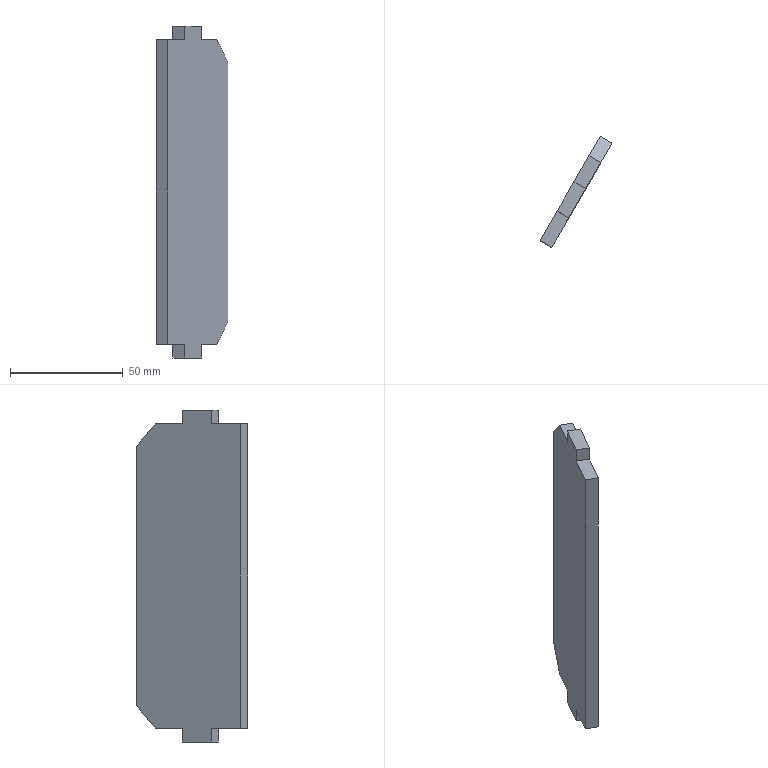Part | SolidWorks | features SMBaseFlange 2, Chamfer 1, FlatPattern 1, SheetMetal 1 | 1 solid | 16 faces | box 31.874 x 49.208 x 147 mm | volume 43699 mm3 | plane 16
STEP:
#1=CARTESIAN_POINT('',(44.488,-29.227,135.));
#2=VERTEX_POINT('',#1);
#3=CARTESIAN_POINT('',(39.291,-26.227,135.));
#4=VERTEX_POINT('',#3);
#5=CARTESIAN_POINT('',(44.488,-29.227,135.));
#6=DIRECTION('',(-0.866,0.5,0.));
#7=VECTOR('',#6,1000.);
#8=LINE('',#5,#7);
#9=EDGE_CURVE('',#2,#4,#8,.T.);
#10=ORIENTED_EDGE('',*,*,#9,.F.);
#11=CARTESIAN_POINT('',(51.166,-17.66,135.));
#12=VERTEX_POINT('',#11);
#13=CARTESIAN_POINT('',(29.488,-55.208,135.));
#14=DIRECTION('',(0.5,0.866,0.));
#15=VECTOR('',#14,1000.);
#16=LINE('',#13,#15);
#17=EDGE_CURVE('',#2,#12,#16,.T.);
#18=ORIENTED_EDGE('',*,*,#17,.T.);
#19=CARTESIAN_POINT('',(45.97,-14.66,135.));
#20=VERTEX_POINT('',#19);
#21=CARTESIAN_POINT('',(45.97,-14.66,135.));
#22=DIRECTION('',(-0.866,0.5,0.));
#23=VECTOR('',#22,1000.);
#24=LINE('',#21,#23);
#25=EDGE_CURVE('',#12,#20,#24,.T.);
#26=ORIENTED_EDGE('',*,*,#25,.T.);
#27=CARTESIAN_POINT('',(24.291,-52.208,135.));
#28=DIRECTION('',(0.5,0.866,0.));
#29=VECTOR('',#28,1000.);
#30=LINE('',#27,#29);
#31=EDGE_CURVE('',#4,#20,#30,.T.);
#32=ORIENTED_EDGE('',*,*,#31,.F.);
#33=EDGE_LOOP('',(#10,#18,#26,#32));
#34=FACE_OUTER_BOUND('',#33,.T.);
#35=CARTESIAN_POINT('',(0.,0.,135.));
#36=DIRECTION('',(0.,0.,-1.));
#37=DIRECTION('',(-1.,0.,0.));
#38=AXIS2_PLACEMENT_3D('',#35,#36,#37);
#39=PLANE('',#38);
#40=ADVANCED_FACE('',(#34),#39,.F.);
#41=CARTESIAN_POINT('',(44.488,-29.227,0.));
#42=VERTEX_POINT('',#41);
#43=CARTESIAN_POINT('',(51.166,-17.66,0.));
#44=VERTEX_POINT('',#43);
#45=CARTESIAN_POINT('',(29.488,-55.208,0.));
#46=DIRECTION('',(0.5,0.866,0.));
#47=VECTOR('',#46,1000.);
#48=LINE('',#45,#47);
#49=EDGE_CURVE('',#42,#44,#48,.T.);
#50=ORIENTED_EDGE('',*,*,#49,.F.);
#51=CARTESIAN_POINT('',(39.291,-26.227,0.));
#52=VERTEX_POINT('',#51);
#53=CARTESIAN_POINT('',(44.488,-29.227,0.));
#54=DIRECTION('',(-0.866,0.5,0.));
#55=VECTOR('',#54,1000.);
#56=LINE('',#53,#55);
#57=EDGE_CURVE('',#42,#52,#56,.T.);
#58=ORIENTED_EDGE('',*,*,#57,.T.);
#59=CARTESIAN_POINT('',(45.97,-14.66,0.));
#60=VERTEX_POINT('',#59);
#61=CARTESIAN_POINT('',(24.291,-52.208,0.));
#62=DIRECTION('',(0.5,0.866,0.));
#63=VECTOR('',#62,1000.);
#64=LINE('',#61,#63);
#65=EDGE_CURVE('',#52,#60,#64,.T.);
#66=ORIENTED_EDGE('',*,*,#65,.T.);
#67=CARTESIAN_POINT('',(5.144,8.91,0.));
#68=DIRECTION('',(0.866,-0.5,0.));
#69=VECTOR('',#68,1000.);
#70=LINE('',#67,#69);
#71=EDGE_CURVE('',#60,#44,#70,.T.);
#72=ORIENTED_EDGE('',*,*,#71,.T.);
#73=EDGE_LOOP('',(#50,#58,#66,#72));
#74=FACE_OUTER_BOUND('',#73,.T.);
#75=CARTESIAN_POINT('',(0.,0.,0.));
#76=DIRECTION('',(0.,0.,-1.));
#77=DIRECTION('',(-1.,0.,0.));
#78=AXIS2_PLACEMENT_3D('',#75,#76,#77);
#79=PLANE('',#78);
#80=ADVANCED_FACE('',(#74),#79,.T.);
#81=CARTESIAN_POINT('',(56.166,-9.,125.));
#82=VERTEX_POINT('',#81);
#83=CARTESIAN_POINT('',(56.166,-9.,10.));
#84=VERTEX_POINT('',#83);
#85=CARTESIAN_POINT('',(56.166,-9.,135.));
#86=DIRECTION('',(0.,0.,-1.));
#87=VECTOR('',#86,1000.);
#88=LINE('',#85,#87);
#89=EDGE_CURVE('',#82,#84,#88,.T.);
#90=ORIENTED_EDGE('',*,*,#89,.F.);
#91=CARTESIAN_POINT('',(56.166,-9.,125.));
#92=DIRECTION('',(-0.3536,-0.6124,0.7071));
#93=VECTOR('',#92,1000.);
#94=LINE('',#91,#93);
#95=EDGE_CURVE('',#82,#12,#94,.T.);
#96=ORIENTED_EDGE('',*,*,#95,.T.);
#97=ORIENTED_EDGE('',*,*,#17,.F.);
#98=CARTESIAN_POINT('',(44.488,-29.227,141.));
#99=VERTEX_POINT('',#98);
#100=CARTESIAN_POINT('',(44.488,-29.227,135.));
#101=DIRECTION('',(0.,0.,-1.));
#102=VECTOR('',#101,1000.);
#103=LINE('',#100,#102);
#104=EDGE_CURVE('',#99,#2,#103,.T.);
#105=ORIENTED_EDGE('',*,*,#104,.F.);
#106=CARTESIAN_POINT('',(36.988,-42.218,141.));
#107=VERTEX_POINT('',#106);
#108=CARTESIAN_POINT('',(44.488,-29.227,141.));
#109=DIRECTION('',(0.5,0.866,0.));
#110=VECTOR('',#109,1000.);
#111=LINE('',#108,#110);
#112=EDGE_CURVE('',#107,#99,#111,.T.);
#113=ORIENTED_EDGE('',*,*,#112,.F.);
#114=CARTESIAN_POINT('',(36.988,-42.218,135.));
#115=VERTEX_POINT('',#114);
#116=CARTESIAN_POINT('',(36.988,-42.218,141.));
#117=DIRECTION('',(0.,0.,1.));
#118=VECTOR('',#117,1000.);
#119=LINE('',#116,#118);
#120=EDGE_CURVE('',#115,#107,#119,.T.);
#121=ORIENTED_EDGE('',*,*,#120,.F.);
#122=CARTESIAN_POINT('',(29.488,-55.208,135.));
#123=VERTEX_POINT('',#122);
#124=CARTESIAN_POINT('',(29.488,-55.208,135.));
#125=DIRECTION('',(0.5,0.866,0.));
#126=VECTOR('',#125,1000.);
#127=LINE('',#124,#126);
#128=EDGE_CURVE('',#123,#115,#127,.T.);
#129=ORIENTED_EDGE('',*,*,#128,.F.);
#130=CARTESIAN_POINT('',(29.488,-55.208,0.));
#131=VERTEX_POINT('',#130);
#132=CARTESIAN_POINT('',(29.488,-55.208,135.));
#133=DIRECTION('',(0.,0.,-1.));
#134=VECTOR('',#133,1000.);
#135=LINE('',#132,#134);
#136=EDGE_CURVE('',#123,#131,#135,.T.);
#137=ORIENTED_EDGE('',*,*,#136,.T.);
#138=CARTESIAN_POINT('',(36.988,-42.218,0.));
#139=VERTEX_POINT('',#138);
#140=CARTESIAN_POINT('',(29.488,-55.208,0.));
#141=DIRECTION('',(0.5,0.866,0.));
#142=VECTOR('',#141,1000.);
#143=LINE('',#140,#142);
#144=EDGE_CURVE('',#131,#139,#143,.T.);
#145=ORIENTED_EDGE('',*,*,#144,.T.);
#146=CARTESIAN_POINT('',(36.988,-42.218,-6.));
#147=VERTEX_POINT('',#146);
#148=CARTESIAN_POINT('',(36.988,-42.218,-6.));
#149=DIRECTION('',(0.,0.,1.));
#150=VECTOR('',#149,1000.);
#151=LINE('',#148,#150);
#152=EDGE_CURVE('',#147,#139,#151,.T.);
#153=ORIENTED_EDGE('',*,*,#152,.F.);
#154=CARTESIAN_POINT('',(44.488,-29.227,-6.));
#155=VERTEX_POINT('',#154);
#156=CARTESIAN_POINT('',(44.488,-29.227,-6.));
#157=DIRECTION('',(-0.5,-0.866,0.));
#158=VECTOR('',#157,1000.);
#159=LINE('',#156,#158);
#160=EDGE_CURVE('',#155,#147,#159,.T.);
#161=ORIENTED_EDGE('',*,*,#160,.F.);
#162=CARTESIAN_POINT('',(44.488,-29.227,0.));
#163=DIRECTION('',(0.,0.,-1.));
#164=VECTOR('',#163,1000.);
#165=LINE('',#162,#164);
#166=EDGE_CURVE('',#42,#155,#165,.T.);
#167=ORIENTED_EDGE('',*,*,#166,.F.);
#168=ORIENTED_EDGE('',*,*,#49,.T.);
#169=CARTESIAN_POINT('',(51.166,-17.66,0.));
#170=DIRECTION('',(0.3536,0.6124,0.7071));
#171=VECTOR('',#170,1000.);
#172=LINE('',#169,#171);
#173=EDGE_CURVE('',#44,#84,#172,.T.);
#174=ORIENTED_EDGE('',*,*,#173,.T.);
#175=EDGE_LOOP('',(#90,#96,#97,#105,#113,#121,#129,#137,#145,#153,#161,#167,#168,#174));
#176=FACE_OUTER_BOUND('',#175,.T.);
#177=CARTESIAN_POINT('',(29.488,-55.208,135.));
#178=DIRECTION('',(-0.866,0.5,0.));
#179=DIRECTION('',(-0.5,-0.866,0.));
#180=AXIS2_PLACEMENT_3D('',#177,#178,#179);
#181=PLANE('',#180);
#182=ADVANCED_FACE('',(#176),#181,.F.);
#183=CARTESIAN_POINT('',(50.97,-6.,125.));
#184=VERTEX_POINT('',#183);
#185=CARTESIAN_POINT('',(50.97,-6.,10.));
#186=VERTEX_POINT('',#185);
#187=CARTESIAN_POINT('',(50.97,-6.,135.));
#188=DIRECTION('',(0.,0.,-1.));
#189=VECTOR('',#188,1000.);
#190=LINE('',#187,#189);
#191=EDGE_CURVE('',#184,#186,#190,.T.);
#192=ORIENTED_EDGE('',*,*,#191,.F.);
#193=CARTESIAN_POINT('',(56.166,-9.,125.));
#194=DIRECTION('',(0.866,-0.5,0.));
#195=VECTOR('',#194,1000.);
#196=LINE('',#193,#195);
#197=EDGE_CURVE('',#184,#82,#196,.T.);
#198=ORIENTED_EDGE('',*,*,#197,.T.);
#199=ORIENTED_EDGE('',*,*,#89,.T.);
#200=CARTESIAN_POINT('',(50.97,-6.,10.));
#201=DIRECTION('',(-0.866,0.5,0.));
#202=VECTOR('',#201,1000.);
#203=LINE('',#200,#202);
#204=EDGE_CURVE('',#84,#186,#203,.T.);
#205=ORIENTED_EDGE('',*,*,#204,.T.);
#206=EDGE_LOOP('',(#192,#198,#199,#205));
#207=FACE_OUTER_BOUND('',#206,.T.);
#208=CARTESIAN_POINT('',(50.97,-6.,135.));
#209=DIRECTION('',(0.5,0.866,0.));
#210=DIRECTION('',(-0.866,0.5,0.));
#211=AXIS2_PLACEMENT_3D('',#208,#209,#210);
#212=PLANE('',#211);
#213=ADVANCED_FACE('',(#207),#212,.T.);
#214=CARTESIAN_POINT('',(24.291,-52.208,135.));
#215=VERTEX_POINT('',#214);
#216=CARTESIAN_POINT('',(31.791,-39.218,135.));
#217=VERTEX_POINT('',#216);
#218=CARTESIAN_POINT('',(24.291,-52.208,135.));
#219=DIRECTION('',(0.5,0.866,0.));
#220=VECTOR('',#219,1000.);
#221=LINE('',#218,#220);
#222=EDGE_CURVE('',#215,#217,#221,.T.);
#223=ORIENTED_EDGE('',*,*,#222,.T.);
#224=CARTESIAN_POINT('',(31.791,-39.218,141.));
#225=VERTEX_POINT('',#224);
#226=CARTESIAN_POINT('',(31.791,-39.218,141.));
#227=DIRECTION('',(0.,0.,1.));
#228=VECTOR('',#227,1000.);
#229=LINE('',#226,#228);
#230=EDGE_CURVE('',#217,#225,#229,.T.);
#231=ORIENTED_EDGE('',*,*,#230,.T.);
#232=CARTESIAN_POINT('',(39.291,-26.227,141.));
#233=VERTEX_POINT('',#232);
#234=CARTESIAN_POINT('',(39.291,-26.227,141.));
#235=DIRECTION('',(0.5,0.866,0.));
#236=VECTOR('',#235,1000.);
#237=LINE('',#234,#236);
#238=EDGE_CURVE('',#225,#233,#237,.T.);
#239=ORIENTED_EDGE('',*,*,#238,.T.);
#240=CARTESIAN_POINT('',(39.291,-26.227,135.));
#241=DIRECTION('',(0.,0.,-1.));
#242=VECTOR('',#241,1000.);
#243=LINE('',#240,#242);
#244=EDGE_CURVE('',#233,#4,#243,.T.);
#245=ORIENTED_EDGE('',*,*,#244,.T.);
#246=ORIENTED_EDGE('',*,*,#31,.T.);
#247=CARTESIAN_POINT('',(35.131,-33.434,156.678));
#248=DIRECTION('',(0.3536,0.6124,-0.7071));
#249=VECTOR('',#248,1000.);
#250=LINE('',#247,#249);
#251=EDGE_CURVE('',#20,#184,#250,.T.);
#252=ORIENTED_EDGE('',*,*,#251,.T.);
#253=ORIENTED_EDGE('',*,*,#191,.T.);
#254=CARTESIAN_POINT('',(68.881,25.023,45.822));
#255=DIRECTION('',(-0.3536,-0.6124,-0.7071));
#256=VECTOR('',#255,1000.);
#257=LINE('',#254,#256);
#258=EDGE_CURVE('',#186,#60,#257,.T.);
#259=ORIENTED_EDGE('',*,*,#258,.T.);
#260=ORIENTED_EDGE('',*,*,#65,.F.);
#261=CARTESIAN_POINT('',(39.291,-26.227,-6.));
#262=VERTEX_POINT('',#261);
#263=CARTESIAN_POINT('',(39.291,-26.227,0.));
#264=DIRECTION('',(0.,0.,-1.));
#265=VECTOR('',#264,1000.);
#266=LINE('',#263,#265);
#267=EDGE_CURVE('',#52,#262,#266,.T.);
#268=ORIENTED_EDGE('',*,*,#267,.T.);
#269=CARTESIAN_POINT('',(31.791,-39.218,-6.));
#270=VERTEX_POINT('',#269);
#271=CARTESIAN_POINT('',(39.291,-26.227,-6.));
#272=DIRECTION('',(-0.5,-0.866,0.));
#273=VECTOR('',#272,1000.);
#274=LINE('',#271,#273);
#275=EDGE_CURVE('',#262,#270,#274,.T.);
#276=ORIENTED_EDGE('',*,*,#275,.T.);
#277=CARTESIAN_POINT('',(31.791,-39.218,0.));
#278=VERTEX_POINT('',#277);
#279=CARTESIAN_POINT('',(31.791,-39.218,-6.));
#280=DIRECTION('',(0.,0.,1.));
#281=VECTOR('',#280,1000.);
#282=LINE('',#279,#281);
#283=EDGE_CURVE('',#270,#278,#282,.T.);
#284=ORIENTED_EDGE('',*,*,#283,.T.);
#285=CARTESIAN_POINT('',(24.291,-52.208,0.));
#286=VERTEX_POINT('',#285);
#287=CARTESIAN_POINT('',(24.291,-52.208,0.));
#288=DIRECTION('',(0.5,0.866,0.));
#289=VECTOR('',#288,1000.);
#290=LINE('',#287,#289);
#291=EDGE_CURVE('',#286,#278,#290,.T.);
#292=ORIENTED_EDGE('',*,*,#291,.F.);
#293=CARTESIAN_POINT('',(24.291,-52.208,135.));
#294=DIRECTION('',(0.,0.,-1.));
#295=VECTOR('',#294,1000.);
#296=LINE('',#293,#295);
#297=EDGE_CURVE('',#215,#286,#296,.T.);
#298=ORIENTED_EDGE('',*,*,#297,.F.);
#299=EDGE_LOOP('',(#223,#231,#239,#245,#246,#252,#253,#259,#260,#268,#276,#284,#292,#298));
#300=FACE_OUTER_BOUND('',#299,.T.);
#301=CARTESIAN_POINT('',(24.291,-52.208,135.));
#302=DIRECTION('',(-0.866,0.5,0.));
#303=DIRECTION('',(-0.5,-0.866,0.));
#304=AXIS2_PLACEMENT_3D('',#301,#302,#303);
#305=PLANE('',#304);
#306=ADVANCED_FACE('',(#300),#305,.T.);
#307=CARTESIAN_POINT('',(29.488,-55.208,0.));
#308=DIRECTION('',(-0.866,0.5,0.));
#309=VECTOR('',#308,1000.);
#310=LINE('',#307,#309);
#311=EDGE_CURVE('',#131,#286,#310,.T.);
#312=ORIENTED_EDGE('',*,*,#311,.F.);
#313=ORIENTED_EDGE('',*,*,#136,.F.);
#314=CARTESIAN_POINT('',(29.488,-55.208,135.));
#315=DIRECTION('',(-0.866,0.5,0.));
#316=VECTOR('',#315,1000.);
#317=LINE('',#314,#316);
#318=EDGE_CURVE('',#123,#215,#317,.T.);
#319=ORIENTED_EDGE('',*,*,#318,.T.);
#320=ORIENTED_EDGE('',*,*,#297,.T.);
#321=EDGE_LOOP('',(#312,#313,#319,#320));
#322=FACE_OUTER_BOUND('',#321,.T.);
#323=CARTESIAN_POINT('',(29.488,-55.208,135.));
#324=DIRECTION('',(-0.5,-0.866,0.));
#325=DIRECTION('',(0.866,-0.5,0.));
#326=AXIS2_PLACEMENT_3D('',#323,#324,#325);
#327=PLANE('',#326);
#328=ADVANCED_FACE('',(#322),#327,.T.);
#329=ORIENTED_EDGE('',*,*,#128,.T.);
#330=CARTESIAN_POINT('',(36.988,-42.218,135.));
#331=DIRECTION('',(-0.866,0.5,0.));
#332=VECTOR('',#331,1000.);
#333=LINE('',#330,#332);
#334=EDGE_CURVE('',#115,#217,#333,.T.);
#335=ORIENTED_EDGE('',*,*,#334,.T.);
#336=ORIENTED_EDGE('',*,*,#222,.F.);
#337=ORIENTED_EDGE('',*,*,#318,.F.);
#338=EDGE_LOOP('',(#329,#335,#336,#337));
#339=FACE_OUTER_BOUND('',#338,.T.);
#340=CARTESIAN_POINT('',(0.,0.,135.));
#341=DIRECTION('',(0.,0.,-1.));
#342=DIRECTION('',(-1.,0.,0.));
#343=AXIS2_PLACEMENT_3D('',#340,#341,#342);
#344=PLANE('',#343);
#345=ADVANCED_FACE('',(#339),#344,.F.);
#346=CARTESIAN_POINT('',(36.988,-42.218,0.));
#347=DIRECTION('',(-0.866,0.5,0.));
#348=VECTOR('',#347,1000.);
#349=LINE('',#346,#348);
#350=EDGE_CURVE('',#139,#278,#349,.T.);
#351=ORIENTED_EDGE('',*,*,#350,.F.);
#352=ORIENTED_EDGE('',*,*,#144,.F.);
#353=ORIENTED_EDGE('',*,*,#311,.T.);
#354=ORIENTED_EDGE('',*,*,#291,.T.);
#355=EDGE_LOOP('',(#351,#352,#353,#354));
#356=FACE_OUTER_BOUND('',#355,.T.);
#357=CARTESIAN_POINT('',(0.,0.,0.));
#358=DIRECTION('',(0.,0.,-1.));
#359=DIRECTION('',(-1.,0.,0.));
#360=AXIS2_PLACEMENT_3D('',#357,#358,#359);
#361=PLANE('',#360);
#362=ADVANCED_FACE('',(#356),#361,.T.);
#363=ORIENTED_EDGE('',*,*,#251,.F.);
#364=ORIENTED_EDGE('',*,*,#25,.F.);
#365=ORIENTED_EDGE('',*,*,#95,.F.);
#366=ORIENTED_EDGE('',*,*,#197,.F.);
#367=EDGE_LOOP('',(#363,#364,#365,#366));
#368=FACE_OUTER_BOUND('',#367,.T.);
#369=CARTESIAN_POINT('',(50.97,-6.,125.));
#370=DIRECTION('',(0.3536,0.6124,0.7071));
#371=DIRECTION('',(-0.866,0.5,0.));
#372=AXIS2_PLACEMENT_3D('',#369,#370,#371);
#373=PLANE('',#372);
#374=ADVANCED_FACE('',(#368),#373,.T.);
#375=ORIENTED_EDGE('',*,*,#258,.F.);
#376=ORIENTED_EDGE('',*,*,#204,.F.);
#377=ORIENTED_EDGE('',*,*,#173,.F.);
#378=ORIENTED_EDGE('',*,*,#71,.F.);
#379=EDGE_LOOP('',(#375,#376,#377,#378));
#380=FACE_OUTER_BOUND('',#379,.T.);
#381=CARTESIAN_POINT('',(5.144,8.91,0.));
#382=DIRECTION('',(-0.3536,-0.6124,0.7071));
#383=DIRECTION('',(0.866,-0.5,0.));
#384=AXIS2_PLACEMENT_3D('',#381,#382,#383);
#385=PLANE('',#384);
#386=ADVANCED_FACE('',(#380),#385,.F.);
#387=ORIENTED_EDGE('',*,*,#283,.F.);
#388=CARTESIAN_POINT('',(36.988,-42.218,-6.));
#389=DIRECTION('',(-0.866,0.5,0.));
#390=VECTOR('',#389,1000.);
#391=LINE('',#388,#390);
#392=EDGE_CURVE('',#147,#270,#391,.T.);
#393=ORIENTED_EDGE('',*,*,#392,.F.);
#394=ORIENTED_EDGE('',*,*,#152,.T.);
#395=ORIENTED_EDGE('',*,*,#350,.T.);
#396=EDGE_LOOP('',(#387,#393,#394,#395));
#397=FACE_OUTER_BOUND('',#396,.T.);
#398=CARTESIAN_POINT('',(36.988,-42.218,-6.));
#399=DIRECTION('',(-0.5,-0.866,0.));
#400=DIRECTION('',(0.866,-0.5,0.));
#401=AXIS2_PLACEMENT_3D('',#398,#399,#400);
#402=PLANE('',#401);
#403=ADVANCED_FACE('',(#397),#402,.T.);
#404=ORIENTED_EDGE('',*,*,#275,.F.);
#405=CARTESIAN_POINT('',(44.488,-29.227,-6.));
#406=DIRECTION('',(-0.866,0.5,0.));
#407=VECTOR('',#406,1000.);
#408=LINE('',#405,#407);
#409=EDGE_CURVE('',#155,#262,#408,.T.);
#410=ORIENTED_EDGE('',*,*,#409,.F.);
#411=ORIENTED_EDGE('',*,*,#160,.T.);
#412=ORIENTED_EDGE('',*,*,#392,.T.);
#413=EDGE_LOOP('',(#404,#410,#411,#412));
#414=FACE_OUTER_BOUND('',#413,.T.);
#415=CARTESIAN_POINT('',(44.488,-29.227,-6.));
#416=DIRECTION('',(0.,0.,-1.));
#417=DIRECTION('',(0.,1.,0.));
#418=AXIS2_PLACEMENT_3D('',#415,#416,#417);
#419=PLANE('',#418);
#420=ADVANCED_FACE('',(#414),#419,.T.);
#421=ORIENTED_EDGE('',*,*,#267,.F.);
#422=ORIENTED_EDGE('',*,*,#57,.F.);
#423=ORIENTED_EDGE('',*,*,#166,.T.);
#424=ORIENTED_EDGE('',*,*,#409,.T.);
#425=EDGE_LOOP('',(#421,#422,#423,#424));
#426=FACE_OUTER_BOUND('',#425,.T.);
#427=CARTESIAN_POINT('',(44.488,-29.227,0.));
#428=DIRECTION('',(0.5,0.866,0.));
#429=DIRECTION('',(-0.866,0.5,0.));
#430=AXIS2_PLACEMENT_3D('',#427,#428,#429);
#431=PLANE('',#430);
#432=ADVANCED_FACE('',(#426),#431,.T.);
#433=ORIENTED_EDGE('',*,*,#244,.F.);
#434=CARTESIAN_POINT('',(44.488,-29.227,141.));
#435=DIRECTION('',(-0.866,0.5,0.));
#436=VECTOR('',#435,1000.);
#437=LINE('',#434,#436);
#438=EDGE_CURVE('',#99,#233,#437,.T.);
#439=ORIENTED_EDGE('',*,*,#438,.F.);
#440=ORIENTED_EDGE('',*,*,#104,.T.);
#441=ORIENTED_EDGE('',*,*,#9,.T.);
#442=EDGE_LOOP('',(#433,#439,#440,#441));
#443=FACE_OUTER_BOUND('',#442,.T.);
#444=CARTESIAN_POINT('',(44.488,-29.227,135.));
#445=DIRECTION('',(0.5,0.866,0.));
#446=DIRECTION('',(-0.866,0.5,0.));
#447=AXIS2_PLACEMENT_3D('',#444,#445,#446);
#448=PLANE('',#447);
#449=ADVANCED_FACE('',(#443),#448,.T.);
#450=ORIENTED_EDGE('',*,*,#238,.F.);
#451=CARTESIAN_POINT('',(36.988,-42.218,141.));
#452=DIRECTION('',(-0.866,0.5,0.));
#453=VECTOR('',#452,1000.);
#454=LINE('',#451,#453);
#455=EDGE_CURVE('',#107,#225,#454,.T.);
#456=ORIENTED_EDGE('',*,*,#455,.F.);
#457=ORIENTED_EDGE('',*,*,#112,.T.);
#458=ORIENTED_EDGE('',*,*,#438,.T.);
#459=EDGE_LOOP('',(#450,#456,#457,#458));
#460=FACE_OUTER_BOUND('',#459,.T.);
#461=CARTESIAN_POINT('',(44.488,-29.227,141.));
#462=DIRECTION('',(0.,0.,1.));
#463=DIRECTION('',(1.,0.,0.));
#464=AXIS2_PLACEMENT_3D('',#461,#462,#463);
#465=PLANE('',#464);
#466=ADVANCED_FACE('',(#460),#465,.T.);
#467=ORIENTED_EDGE('',*,*,#230,.F.);
#468=ORIENTED_EDGE('',*,*,#334,.F.);
#469=ORIENTED_EDGE('',*,*,#120,.T.);
#470=ORIENTED_EDGE('',*,*,#455,.T.);
#471=EDGE_LOOP('',(#467,#468,#469,#470));
#472=FACE_OUTER_BOUND('',#471,.T.);
#473=CARTESIAN_POINT('',(36.988,-42.218,141.));
#474=DIRECTION('',(-0.5,-0.866,0.));
#475=DIRECTION('',(0.866,-0.5,0.));
#476=AXIS2_PLACEMENT_3D('',#473,#474,#475);
#477=PLANE('',#476);
#478=ADVANCED_FACE('',(#472),#477,.T.);
#479=CLOSED_SHELL('',(#40,#80,#182,#213,#306,#328,#345,#362,#374,#386,#403,#420,#432,#449,#466,#478));
#480=MANIFOLD_SOLID_BREP('',#479);
#481=CARTESIAN_POINT('',(0.,0.,0.));
#482=DIRECTION('',(0.,0.,1.));
#483=DIRECTION('',(1.,0.,0.));
#484=AXIS2_PLACEMENT_3D('',#481,#482,#483);
#485=(LENGTH_UNIT()NAMED_UNIT(*)SI_UNIT(.MILLI.,.METRE.));
#486=UNCERTAINTY_MEASURE_WITH_UNIT(LENGTH_MEASURE(0.00001),#485,'','');
#487=(NAMED_UNIT(*)PLANE_ANGLE_UNIT()SI_UNIT($,.RADIAN.));
#488=(NAMED_UNIT(*)SI_UNIT($,.STERADIAN.)SOLID_ANGLE_UNIT());
#489=(GEOMETRIC_REPRESENTATION_CONTEXT(3)GLOBAL_UNCERTAINTY_ASSIGNED_CONTEXT((#486))GLOBAL_UNIT_ASSIGNED_CONTEXT((#485,#487,#488))REPRESENTATION_CONTEXT('',''));
#490=ADVANCED_BREP_SHAPE_REPRESENTATION('',(#480,#484),#489);